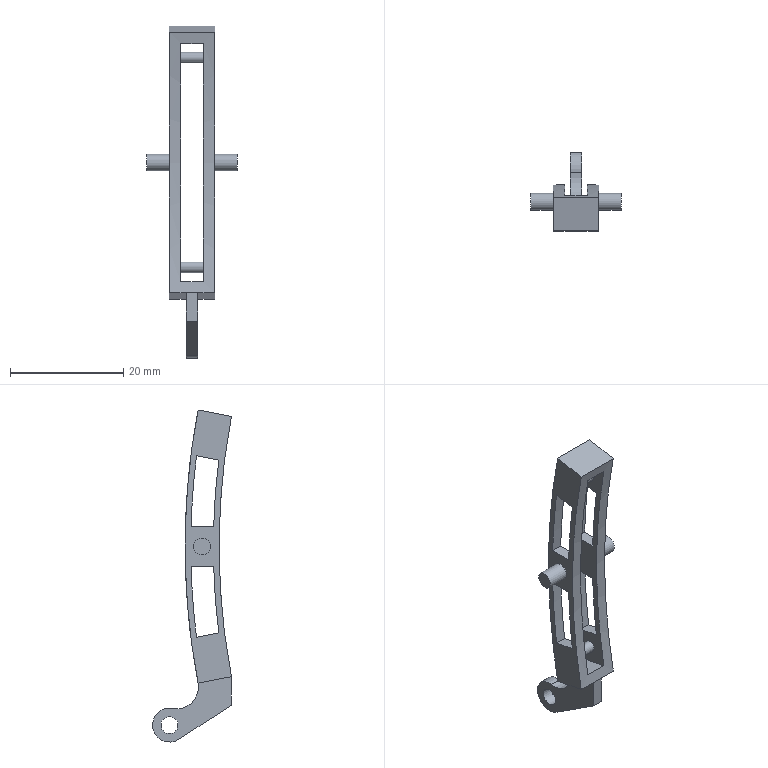Part | STEP file | 2-14 | 1 solid | 40 faces | box 16 x 13.946 x 58.697 mm | volume 1069 mm3 | plane 23 | cylinder 17 | commonest cylinder face diameters 246 x4 254 x4 3 x3 2 x2 6 x1 7.668 x1